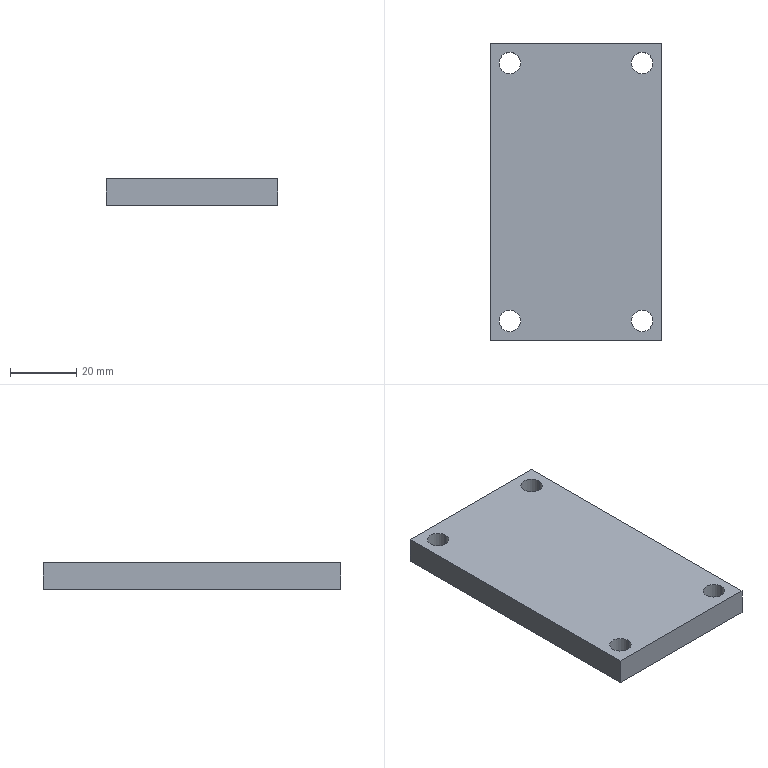Part | STEP file | X77-04017 | 1 solid | 14 faces | box 52 x 90 x 8 mm | volume 36378 mm3 | cylinder 8 | plane 6 | commonest cylinder face diameters 6.5 x8
STEP:
#1=CARTESIAN_POINT('',(16.75,-39.,8.));
#2=VERTEX_POINT('',#1);
#3=CARTESIAN_POINT('',(23.25,-39.,8.));
#4=VERTEX_POINT('',#3);
#5=CARTESIAN_POINT('',(20.,-39.,8.));
#6=DIRECTION('',(0.,0.,1.));
#7=DIRECTION('',(1.,0.,0.));
#8=AXIS2_PLACEMENT_3D('',#5,#6,#7);
#9=CIRCLE('',#8,3.25);
#10=EDGE_CURVE('',#2,#4,#9,.T.);
#11=ORIENTED_EDGE('',*,*,#10,.T.);
#12=CARTESIAN_POINT('',(23.25,-39.,0.));
#13=VERTEX_POINT('',#12);
#14=CARTESIAN_POINT('',(23.25,-39.,8.));
#15=DIRECTION('',(0.,0.,-1.));
#16=VECTOR('',#15,1000.);
#17=LINE('',#14,#16);
#18=EDGE_CURVE('',#4,#13,#17,.T.);
#19=ORIENTED_EDGE('',*,*,#18,.T.);
#20=CARTESIAN_POINT('',(16.75,-39.,0.));
#21=VERTEX_POINT('',#20);
#22=CARTESIAN_POINT('',(20.,-39.,0.));
#23=DIRECTION('',(0.,0.,1.));
#24=DIRECTION('',(1.,0.,0.));
#25=AXIS2_PLACEMENT_3D('',#22,#23,#24);
#26=CIRCLE('',#25,3.25);
#27=EDGE_CURVE('',#21,#13,#26,.T.);
#28=ORIENTED_EDGE('',*,*,#27,.F.);
#29=CARTESIAN_POINT('',(16.75,-39.,8.));
#30=DIRECTION('',(0.,0.,-1.));
#31=VECTOR('',#30,1000.);
#32=LINE('',#29,#31);
#33=EDGE_CURVE('',#2,#21,#32,.T.);
#34=ORIENTED_EDGE('',*,*,#33,.F.);
#35=EDGE_LOOP('',(#11,#19,#28,#34));
#36=FACE_OUTER_BOUND('',#35,.T.);
#37=CARTESIAN_POINT('',(20.,-39.,8.));
#38=DIRECTION('',(0.,0.,-1.));
#39=DIRECTION('',(-1.,0.,0.));
#40=AXIS2_PLACEMENT_3D('',#37,#38,#39);
#41=CYLINDRICAL_SURFACE('',#40,3.25);
#42=ADVANCED_FACE('',(#36),#41,.F.);
#43=CARTESIAN_POINT('',(-23.25,-39.,8.));
#44=VERTEX_POINT('',#43);
#45=CARTESIAN_POINT('',(-16.75,-39.,8.));
#46=VERTEX_POINT('',#45);
#47=CARTESIAN_POINT('',(-20.,-39.,8.));
#48=DIRECTION('',(0.,0.,1.));
#49=DIRECTION('',(1.,0.,0.));
#50=AXIS2_PLACEMENT_3D('',#47,#48,#49);
#51=CIRCLE('',#50,3.25);
#52=EDGE_CURVE('',#44,#46,#51,.T.);
#53=ORIENTED_EDGE('',*,*,#52,.T.);
#54=CARTESIAN_POINT('',(-16.75,-39.,0.));
#55=VERTEX_POINT('',#54);
#56=CARTESIAN_POINT('',(-16.75,-39.,8.));
#57=DIRECTION('',(0.,0.,-1.));
#58=VECTOR('',#57,1000.);
#59=LINE('',#56,#58);
#60=EDGE_CURVE('',#46,#55,#59,.T.);
#61=ORIENTED_EDGE('',*,*,#60,.T.);
#62=CARTESIAN_POINT('',(-23.25,-39.,0.));
#63=VERTEX_POINT('',#62);
#64=CARTESIAN_POINT('',(-20.,-39.,0.));
#65=DIRECTION('',(0.,0.,1.));
#66=DIRECTION('',(1.,0.,0.));
#67=AXIS2_PLACEMENT_3D('',#64,#65,#66);
#68=CIRCLE('',#67,3.25);
#69=EDGE_CURVE('',#63,#55,#68,.T.);
#70=ORIENTED_EDGE('',*,*,#69,.F.);
#71=CARTESIAN_POINT('',(-23.25,-39.,8.));
#72=DIRECTION('',(0.,0.,-1.));
#73=VECTOR('',#72,1000.);
#74=LINE('',#71,#73);
#75=EDGE_CURVE('',#44,#63,#74,.T.);
#76=ORIENTED_EDGE('',*,*,#75,.F.);
#77=EDGE_LOOP('',(#53,#61,#70,#76));
#78=FACE_OUTER_BOUND('',#77,.T.);
#79=CARTESIAN_POINT('',(-20.,-39.,8.));
#80=DIRECTION('',(0.,0.,-1.));
#81=DIRECTION('',(-1.,0.,0.));
#82=AXIS2_PLACEMENT_3D('',#79,#80,#81);
#83=CYLINDRICAL_SURFACE('',#82,3.25);
#84=ADVANCED_FACE('',(#78),#83,.F.);
#85=CARTESIAN_POINT('',(-23.25,39.,8.));
#86=VERTEX_POINT('',#85);
#87=CARTESIAN_POINT('',(-16.75,39.,8.));
#88=VERTEX_POINT('',#87);
#89=CARTESIAN_POINT('',(-20.,39.,8.));
#90=DIRECTION('',(0.,0.,1.));
#91=DIRECTION('',(1.,0.,0.));
#92=AXIS2_PLACEMENT_3D('',#89,#90,#91);
#93=CIRCLE('',#92,3.25);
#94=EDGE_CURVE('',#86,#88,#93,.T.);
#95=ORIENTED_EDGE('',*,*,#94,.T.);
#96=CARTESIAN_POINT('',(-16.75,39.,0.));
#97=VERTEX_POINT('',#96);
#98=CARTESIAN_POINT('',(-16.75,39.,8.));
#99=DIRECTION('',(0.,0.,-1.));
#100=VECTOR('',#99,1000.);
#101=LINE('',#98,#100);
#102=EDGE_CURVE('',#88,#97,#101,.T.);
#103=ORIENTED_EDGE('',*,*,#102,.T.);
#104=CARTESIAN_POINT('',(-23.25,39.,0.));
#105=VERTEX_POINT('',#104);
#106=CARTESIAN_POINT('',(-20.,39.,0.));
#107=DIRECTION('',(0.,0.,1.));
#108=DIRECTION('',(1.,0.,0.));
#109=AXIS2_PLACEMENT_3D('',#106,#107,#108);
#110=CIRCLE('',#109,3.25);
#111=EDGE_CURVE('',#105,#97,#110,.T.);
#112=ORIENTED_EDGE('',*,*,#111,.F.);
#113=CARTESIAN_POINT('',(-23.25,39.,8.));
#114=DIRECTION('',(0.,0.,-1.));
#115=VECTOR('',#114,1000.);
#116=LINE('',#113,#115);
#117=EDGE_CURVE('',#86,#105,#116,.T.);
#118=ORIENTED_EDGE('',*,*,#117,.F.);
#119=EDGE_LOOP('',(#95,#103,#112,#118));
#120=FACE_OUTER_BOUND('',#119,.T.);
#121=CARTESIAN_POINT('',(-20.,39.,8.));
#122=DIRECTION('',(0.,0.,-1.));
#123=DIRECTION('',(-1.,0.,0.));
#124=AXIS2_PLACEMENT_3D('',#121,#122,#123);
#125=CYLINDRICAL_SURFACE('',#124,3.25);
#126=ADVANCED_FACE('',(#120),#125,.F.);
#127=CARTESIAN_POINT('',(16.75,39.,8.));
#128=VERTEX_POINT('',#127);
#129=CARTESIAN_POINT('',(23.25,39.,8.));
#130=VERTEX_POINT('',#129);
#131=CARTESIAN_POINT('',(20.,39.,8.));
#132=DIRECTION('',(0.,0.,1.));
#133=DIRECTION('',(1.,0.,0.));
#134=AXIS2_PLACEMENT_3D('',#131,#132,#133);
#135=CIRCLE('',#134,3.25);
#136=EDGE_CURVE('',#128,#130,#135,.T.);
#137=ORIENTED_EDGE('',*,*,#136,.T.);
#138=CARTESIAN_POINT('',(23.25,39.,0.));
#139=VERTEX_POINT('',#138);
#140=CARTESIAN_POINT('',(23.25,39.,8.));
#141=DIRECTION('',(0.,0.,-1.));
#142=VECTOR('',#141,1000.);
#143=LINE('',#140,#142);
#144=EDGE_CURVE('',#130,#139,#143,.T.);
#145=ORIENTED_EDGE('',*,*,#144,.T.);
#146=CARTESIAN_POINT('',(16.75,39.,0.));
#147=VERTEX_POINT('',#146);
#148=CARTESIAN_POINT('',(20.,39.,0.));
#149=DIRECTION('',(0.,0.,1.));
#150=DIRECTION('',(1.,0.,0.));
#151=AXIS2_PLACEMENT_3D('',#148,#149,#150);
#152=CIRCLE('',#151,3.25);
#153=EDGE_CURVE('',#147,#139,#152,.T.);
#154=ORIENTED_EDGE('',*,*,#153,.F.);
#155=CARTESIAN_POINT('',(16.75,39.,8.));
#156=DIRECTION('',(0.,0.,-1.));
#157=VECTOR('',#156,1000.);
#158=LINE('',#155,#157);
#159=EDGE_CURVE('',#128,#147,#158,.T.);
#160=ORIENTED_EDGE('',*,*,#159,.F.);
#161=EDGE_LOOP('',(#137,#145,#154,#160));
#162=FACE_OUTER_BOUND('',#161,.T.);
#163=CARTESIAN_POINT('',(20.,39.,8.));
#164=DIRECTION('',(0.,0.,-1.));
#165=DIRECTION('',(-1.,0.,0.));
#166=AXIS2_PLACEMENT_3D('',#163,#164,#165);
#167=CYLINDRICAL_SURFACE('',#166,3.25);
#168=ADVANCED_FACE('',(#162),#167,.F.);
#169=ORIENTED_EDGE('',*,*,#52,.F.);
#170=CARTESIAN_POINT('',(-20.,-39.,8.));
#171=DIRECTION('',(0.,0.,1.));
#172=DIRECTION('',(1.,0.,0.));
#173=AXIS2_PLACEMENT_3D('',#170,#171,#172);
#174=CIRCLE('',#173,3.25);
#175=EDGE_CURVE('',#46,#44,#174,.T.);
#176=ORIENTED_EDGE('',*,*,#175,.F.);
#177=EDGE_LOOP('',(#169,#176));
#178=FACE_BOUND('',#177,.T.);
#179=ORIENTED_EDGE('',*,*,#136,.F.);
#180=CARTESIAN_POINT('',(20.,39.,8.));
#181=DIRECTION('',(0.,0.,1.));
#182=DIRECTION('',(1.,0.,0.));
#183=AXIS2_PLACEMENT_3D('',#180,#181,#182);
#184=CIRCLE('',#183,3.25);
#185=EDGE_CURVE('',#130,#128,#184,.T.);
#186=ORIENTED_EDGE('',*,*,#185,.F.);
#187=EDGE_LOOP('',(#179,#186));
#188=FACE_BOUND('',#187,.T.);
#189=CARTESIAN_POINT('',(-26.,45.,8.));
#190=VERTEX_POINT('',#189);
#191=CARTESIAN_POINT('',(-26.,-45.,8.));
#192=VERTEX_POINT('',#191);
#193=CARTESIAN_POINT('',(-26.,-45.,8.));
#194=DIRECTION('',(0.,-1.,0.));
#195=VECTOR('',#194,1000.);
#196=LINE('',#193,#195);
#197=EDGE_CURVE('',#190,#192,#196,.T.);
#198=ORIENTED_EDGE('',*,*,#197,.T.);
#199=CARTESIAN_POINT('',(26.,-45.,8.));
#200=VERTEX_POINT('',#199);
#201=CARTESIAN_POINT('',(-26.,-45.,8.));
#202=DIRECTION('',(1.,0.,0.));
#203=VECTOR('',#202,1000.);
#204=LINE('',#201,#203);
#205=EDGE_CURVE('',#192,#200,#204,.T.);
#206=ORIENTED_EDGE('',*,*,#205,.T.);
#207=CARTESIAN_POINT('',(26.,45.,8.));
#208=VERTEX_POINT('',#207);
#209=CARTESIAN_POINT('',(26.,-45.,8.));
#210=DIRECTION('',(0.,1.,0.));
#211=VECTOR('',#210,1000.);
#212=LINE('',#209,#211);
#213=EDGE_CURVE('',#200,#208,#212,.T.);
#214=ORIENTED_EDGE('',*,*,#213,.T.);
#215=CARTESIAN_POINT('',(-26.,45.,8.));
#216=DIRECTION('',(-1.,0.,0.));
#217=VECTOR('',#216,1000.);
#218=LINE('',#215,#217);
#219=EDGE_CURVE('',#208,#190,#218,.T.);
#220=ORIENTED_EDGE('',*,*,#219,.T.);
#221=EDGE_LOOP('',(#198,#206,#214,#220));
#222=FACE_OUTER_BOUND('',#221,.T.);
#223=ORIENTED_EDGE('',*,*,#94,.F.);
#224=CARTESIAN_POINT('',(-20.,39.,8.));
#225=DIRECTION('',(0.,0.,1.));
#226=DIRECTION('',(1.,0.,0.));
#227=AXIS2_PLACEMENT_3D('',#224,#225,#226);
#228=CIRCLE('',#227,3.25);
#229=EDGE_CURVE('',#88,#86,#228,.T.);
#230=ORIENTED_EDGE('',*,*,#229,.F.);
#231=EDGE_LOOP('',(#223,#230));
#232=FACE_BOUND('',#231,.T.);
#233=ORIENTED_EDGE('',*,*,#10,.F.);
#234=CARTESIAN_POINT('',(20.,-39.,8.));
#235=DIRECTION('',(0.,0.,1.));
#236=DIRECTION('',(1.,0.,0.));
#237=AXIS2_PLACEMENT_3D('',#234,#235,#236);
#238=CIRCLE('',#237,3.25);
#239=EDGE_CURVE('',#4,#2,#238,.T.);
#240=ORIENTED_EDGE('',*,*,#239,.F.);
#241=EDGE_LOOP('',(#233,#240));
#242=FACE_BOUND('',#241,.T.);
#243=CARTESIAN_POINT('',(-26.,45.,8.));
#244=DIRECTION('',(0.,0.,-1.));
#245=DIRECTION('',(-1.,0.,0.));
#246=AXIS2_PLACEMENT_3D('',#243,#244,#245);
#247=PLANE('',#246);
#248=ADVANCED_FACE('',(#178,#188,#222,#232,#242),#247,.F.);
#249=ORIENTED_EDGE('',*,*,#69,.T.);
#250=CARTESIAN_POINT('',(-20.,-39.,0.));
#251=DIRECTION('',(0.,0.,1.));
#252=DIRECTION('',(1.,0.,0.));
#253=AXIS2_PLACEMENT_3D('',#250,#251,#252);
#254=CIRCLE('',#253,3.25);
#255=EDGE_CURVE('',#55,#63,#254,.T.);
#256=ORIENTED_EDGE('',*,*,#255,.T.);
#257=EDGE_LOOP('',(#249,#256));
#258=FACE_BOUND('',#257,.T.);
#259=ORIENTED_EDGE('',*,*,#153,.T.);
#260=CARTESIAN_POINT('',(20.,39.,0.));
#261=DIRECTION('',(0.,0.,1.));
#262=DIRECTION('',(1.,0.,0.));
#263=AXIS2_PLACEMENT_3D('',#260,#261,#262);
#264=CIRCLE('',#263,3.25);
#265=EDGE_CURVE('',#139,#147,#264,.T.);
#266=ORIENTED_EDGE('',*,*,#265,.T.);
#267=EDGE_LOOP('',(#259,#266));
#268=FACE_BOUND('',#267,.T.);
#269=CARTESIAN_POINT('',(-26.,45.,0.));
#270=VERTEX_POINT('',#269);
#271=CARTESIAN_POINT('',(-26.,-45.,0.));
#272=VERTEX_POINT('',#271);
#273=CARTESIAN_POINT('',(-26.,-45.,0.));
#274=DIRECTION('',(0.,-1.,0.));
#275=VECTOR('',#274,1000.);
#276=LINE('',#273,#275);
#277=EDGE_CURVE('',#270,#272,#276,.T.);
#278=ORIENTED_EDGE('',*,*,#277,.F.);
#279=CARTESIAN_POINT('',(26.,45.,0.));
#280=VERTEX_POINT('',#279);
#281=CARTESIAN_POINT('',(-26.,45.,0.));
#282=DIRECTION('',(-1.,0.,0.));
#283=VECTOR('',#282,1000.);
#284=LINE('',#281,#283);
#285=EDGE_CURVE('',#280,#270,#284,.T.);
#286=ORIENTED_EDGE('',*,*,#285,.F.);
#287=CARTESIAN_POINT('',(26.,-45.,0.));
#288=VERTEX_POINT('',#287);
#289=CARTESIAN_POINT('',(26.,-45.,0.));
#290=DIRECTION('',(0.,1.,0.));
#291=VECTOR('',#290,1000.);
#292=LINE('',#289,#291);
#293=EDGE_CURVE('',#288,#280,#292,.T.);
#294=ORIENTED_EDGE('',*,*,#293,.F.);
#295=CARTESIAN_POINT('',(-26.,-45.,0.));
#296=DIRECTION('',(1.,0.,0.));
#297=VECTOR('',#296,1000.);
#298=LINE('',#295,#297);
#299=EDGE_CURVE('',#272,#288,#298,.T.);
#300=ORIENTED_EDGE('',*,*,#299,.F.);
#301=EDGE_LOOP('',(#278,#286,#294,#300));
#302=FACE_OUTER_BOUND('',#301,.T.);
#303=ORIENTED_EDGE('',*,*,#111,.T.);
#304=CARTESIAN_POINT('',(-20.,39.,0.));
#305=DIRECTION('',(0.,0.,1.));
#306=DIRECTION('',(1.,0.,0.));
#307=AXIS2_PLACEMENT_3D('',#304,#305,#306);
#308=CIRCLE('',#307,3.25);
#309=EDGE_CURVE('',#97,#105,#308,.T.);
#310=ORIENTED_EDGE('',*,*,#309,.T.);
#311=EDGE_LOOP('',(#303,#310));
#312=FACE_BOUND('',#311,.T.);
#313=ORIENTED_EDGE('',*,*,#27,.T.);
#314=CARTESIAN_POINT('',(20.,-39.,0.));
#315=DIRECTION('',(0.,0.,1.));
#316=DIRECTION('',(1.,0.,0.));
#317=AXIS2_PLACEMENT_3D('',#314,#315,#316);
#318=CIRCLE('',#317,3.25);
#319=EDGE_CURVE('',#13,#21,#318,.T.);
#320=ORIENTED_EDGE('',*,*,#319,.T.);
#321=EDGE_LOOP('',(#313,#320));
#322=FACE_BOUND('',#321,.T.);
#323=CARTESIAN_POINT('',(-26.,45.,0.));
#324=DIRECTION('',(0.,0.,-1.));
#325=DIRECTION('',(-1.,0.,0.));
#326=AXIS2_PLACEMENT_3D('',#323,#324,#325);
#327=PLANE('',#326);
#328=ADVANCED_FACE('',(#258,#268,#302,#312,#322),#327,.T.);
#329=ORIENTED_EDGE('',*,*,#277,.T.);
#330=CARTESIAN_POINT('',(-26.,-45.,8.));
#331=DIRECTION('',(0.,0.,-1.));
#332=VECTOR('',#331,1000.);
#333=LINE('',#330,#332);
#334=EDGE_CURVE('',#192,#272,#333,.T.);
#335=ORIENTED_EDGE('',*,*,#334,.F.);
#336=ORIENTED_EDGE('',*,*,#197,.F.);
#337=CARTESIAN_POINT('',(-26.,45.,8.));
#338=DIRECTION('',(0.,0.,-1.));
#339=VECTOR('',#338,1000.);
#340=LINE('',#337,#339);
#341=EDGE_CURVE('',#190,#270,#340,.T.);
#342=ORIENTED_EDGE('',*,*,#341,.T.);
#343=EDGE_LOOP('',(#329,#335,#336,#342));
#344=FACE_OUTER_BOUND('',#343,.T.);
#345=CARTESIAN_POINT('',(-26.,-45.,8.));
#346=DIRECTION('',(1.,0.,0.));
#347=DIRECTION('',(0.,0.,-1.));
#348=AXIS2_PLACEMENT_3D('',#345,#346,#347);
#349=PLANE('',#348);
#350=ADVANCED_FACE('',(#344),#349,.F.);
#351=ORIENTED_EDGE('',*,*,#299,.T.);
#352=CARTESIAN_POINT('',(26.,-45.,8.));
#353=DIRECTION('',(0.,0.,-1.));
#354=VECTOR('',#353,1000.);
#355=LINE('',#352,#354);
#356=EDGE_CURVE('',#200,#288,#355,.T.);
#357=ORIENTED_EDGE('',*,*,#356,.F.);
#358=ORIENTED_EDGE('',*,*,#205,.F.);
#359=ORIENTED_EDGE('',*,*,#334,.T.);
#360=EDGE_LOOP('',(#351,#357,#358,#359));
#361=FACE_OUTER_BOUND('',#360,.T.);
#362=CARTESIAN_POINT('',(-26.,-45.,8.));
#363=DIRECTION('',(0.,1.,0.));
#364=DIRECTION('',(0.,0.,1.));
#365=AXIS2_PLACEMENT_3D('',#362,#363,#364);
#366=PLANE('',#365);
#367=ADVANCED_FACE('',(#361),#366,.F.);
#368=ORIENTED_EDGE('',*,*,#293,.T.);
#369=CARTESIAN_POINT('',(26.,45.,8.));
#370=DIRECTION('',(0.,0.,-1.));
#371=VECTOR('',#370,1000.);
#372=LINE('',#369,#371);
#373=EDGE_CURVE('',#208,#280,#372,.T.);
#374=ORIENTED_EDGE('',*,*,#373,.F.);
#375=ORIENTED_EDGE('',*,*,#213,.F.);
#376=ORIENTED_EDGE('',*,*,#356,.T.);
#377=EDGE_LOOP('',(#368,#374,#375,#376));
#378=FACE_OUTER_BOUND('',#377,.T.);
#379=CARTESIAN_POINT('',(26.,-45.,8.));
#380=DIRECTION('',(-1.,0.,0.));
#381=DIRECTION('',(0.,0.,1.));
#382=AXIS2_PLACEMENT_3D('',#379,#380,#381);
#383=PLANE('',#382);
#384=ADVANCED_FACE('',(#378),#383,.F.);
#385=ORIENTED_EDGE('',*,*,#285,.T.);
#386=ORIENTED_EDGE('',*,*,#341,.F.);
#387=ORIENTED_EDGE('',*,*,#219,.F.);
#388=ORIENTED_EDGE('',*,*,#373,.T.);
#389=EDGE_LOOP('',(#385,#386,#387,#388));
#390=FACE_OUTER_BOUND('',#389,.T.);
#391=CARTESIAN_POINT('',(-26.,45.,8.));
#392=DIRECTION('',(0.,-1.,0.));
#393=DIRECTION('',(1.,0.,0.));
#394=AXIS2_PLACEMENT_3D('',#391,#392,#393);
#395=PLANE('',#394);
#396=ADVANCED_FACE('',(#390),#395,.F.);
#397=ORIENTED_EDGE('',*,*,#144,.F.);
#398=ORIENTED_EDGE('',*,*,#185,.T.);
#399=ORIENTED_EDGE('',*,*,#159,.T.);
#400=ORIENTED_EDGE('',*,*,#265,.F.);
#401=EDGE_LOOP('',(#397,#398,#399,#400));
#402=FACE_OUTER_BOUND('',#401,.T.);
#403=CARTESIAN_POINT('',(20.,39.,8.));
#404=DIRECTION('',(0.,0.,-1.));
#405=DIRECTION('',(-1.,0.,0.));
#406=AXIS2_PLACEMENT_3D('',#403,#404,#405);
#407=CYLINDRICAL_SURFACE('',#406,3.25);
#408=ADVANCED_FACE('',(#402),#407,.F.);
#409=ORIENTED_EDGE('',*,*,#102,.F.);
#410=ORIENTED_EDGE('',*,*,#229,.T.);
#411=ORIENTED_EDGE('',*,*,#117,.T.);
#412=ORIENTED_EDGE('',*,*,#309,.F.);
#413=EDGE_LOOP('',(#409,#410,#411,#412));
#414=FACE_OUTER_BOUND('',#413,.T.);
#415=CARTESIAN_POINT('',(-20.,39.,8.));
#416=DIRECTION('',(0.,0.,-1.));
#417=DIRECTION('',(-1.,0.,0.));
#418=AXIS2_PLACEMENT_3D('',#415,#416,#417);
#419=CYLINDRICAL_SURFACE('',#418,3.25);
#420=ADVANCED_FACE('',(#414),#419,.F.);
#421=ORIENTED_EDGE('',*,*,#60,.F.);
#422=ORIENTED_EDGE('',*,*,#175,.T.);
#423=ORIENTED_EDGE('',*,*,#75,.T.);
#424=ORIENTED_EDGE('',*,*,#255,.F.);
#425=EDGE_LOOP('',(#421,#422,#423,#424));
#426=FACE_OUTER_BOUND('',#425,.T.);
#427=CARTESIAN_POINT('',(-20.,-39.,8.));
#428=DIRECTION('',(0.,0.,-1.));
#429=DIRECTION('',(-1.,0.,0.));
#430=AXIS2_PLACEMENT_3D('',#427,#428,#429);
#431=CYLINDRICAL_SURFACE('',#430,3.25);
#432=ADVANCED_FACE('',(#426),#431,.F.);
#433=ORIENTED_EDGE('',*,*,#18,.F.);
#434=ORIENTED_EDGE('',*,*,#239,.T.);
#435=ORIENTED_EDGE('',*,*,#33,.T.);
#436=ORIENTED_EDGE('',*,*,#319,.F.);
#437=EDGE_LOOP('',(#433,#434,#435,#436));
#438=FACE_OUTER_BOUND('',#437,.T.);
#439=CARTESIAN_POINT('',(20.,-39.,8.));
#440=DIRECTION('',(0.,0.,-1.));
#441=DIRECTION('',(-1.,0.,0.));
#442=AXIS2_PLACEMENT_3D('',#439,#440,#441);
#443=CYLINDRICAL_SURFACE('',#442,3.25);
#444=ADVANCED_FACE('',(#438),#443,.F.);
#445=CLOSED_SHELL('',(#42,#84,#126,#168,#248,#328,#350,#367,#384,#396,#408,#420,#432,#444));
#446=MANIFOLD_SOLID_BREP('',#445);
#447=CARTESIAN_POINT('',(0.,0.,0.));
#448=DIRECTION('',(0.,0.,1.));
#449=DIRECTION('',(1.,0.,0.));
#450=AXIS2_PLACEMENT_3D('',#447,#448,#449);
#451=(LENGTH_UNIT()NAMED_UNIT(*)SI_UNIT(.MILLI.,.METRE.));
#452=UNCERTAINTY_MEASURE_WITH_UNIT(LENGTH_MEASURE(0.00001),#451,'','');
#453=(NAMED_UNIT(*)PLANE_ANGLE_UNIT()SI_UNIT($,.RADIAN.));
#454=(NAMED_UNIT(*)SI_UNIT($,.STERADIAN.)SOLID_ANGLE_UNIT());
#455=(GEOMETRIC_REPRESENTATION_CONTEXT(3)GLOBAL_UNCERTAINTY_ASSIGNED_CONTEXT((#452))GLOBAL_UNIT_ASSIGNED_CONTEXT((#451,#453,#454))REPRESENTATION_CONTEXT('',''));
#456=ADVANCED_BREP_SHAPE_REPRESENTATION('',(#446,#450),#455);